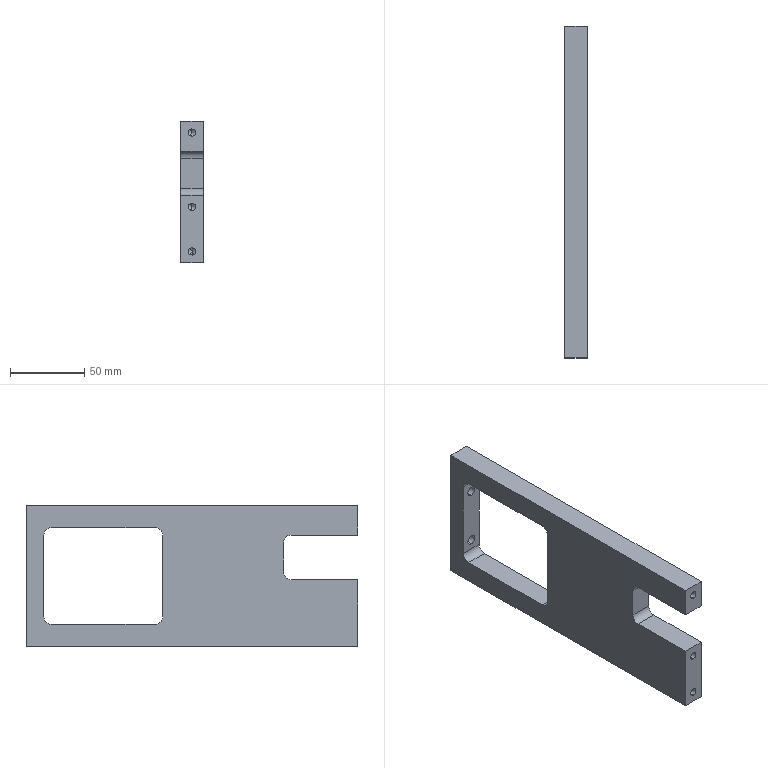Part | SolidWorks | features HoleWzd 5, Cut 1, Extrusion 1 | 1 solid | 60 faces | box 15 x 223.5 x 95 mm | volume 215829 mm3 | cylinder 28 | cone 18 | plane 14 | commonest cylinder face diameters 5 x10 4.2 x8 10 x6 6.6 x4